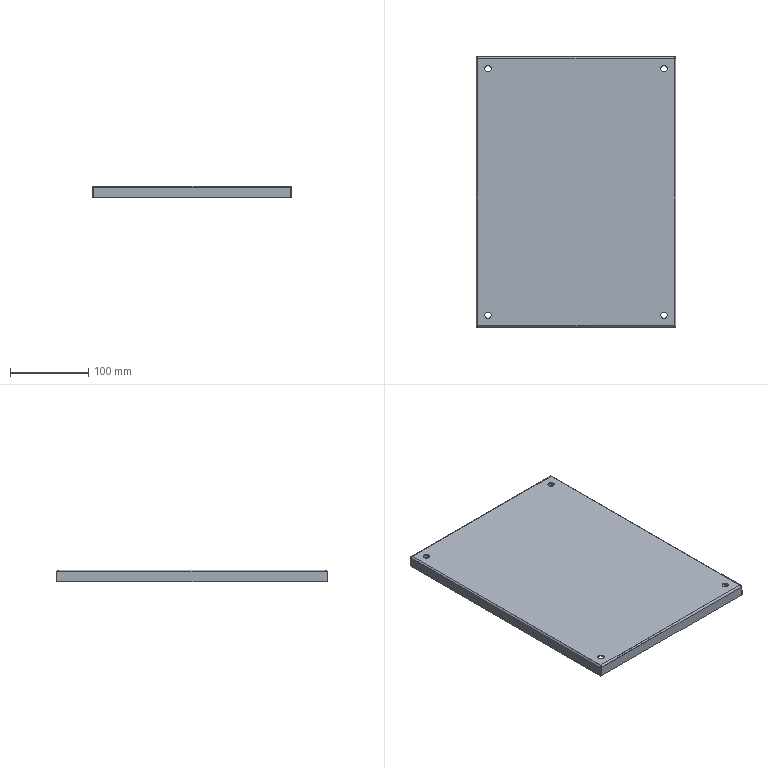Part | SolidWorks | features CornerFeat 1, Cut 1, EdgeFlange 1, FlatPattern 1, MoveCopyBody 1, SMBaseFlange 1, SheetMetal 1 | 1 solid | 46 faces | box 254.629 x 344.629 x 15 mm | volume 123831 mm3 | plane 22 | cylinder 16 | spline 8 | commonest cylinder face diameters 8 x8 2 x4 4.4 x4